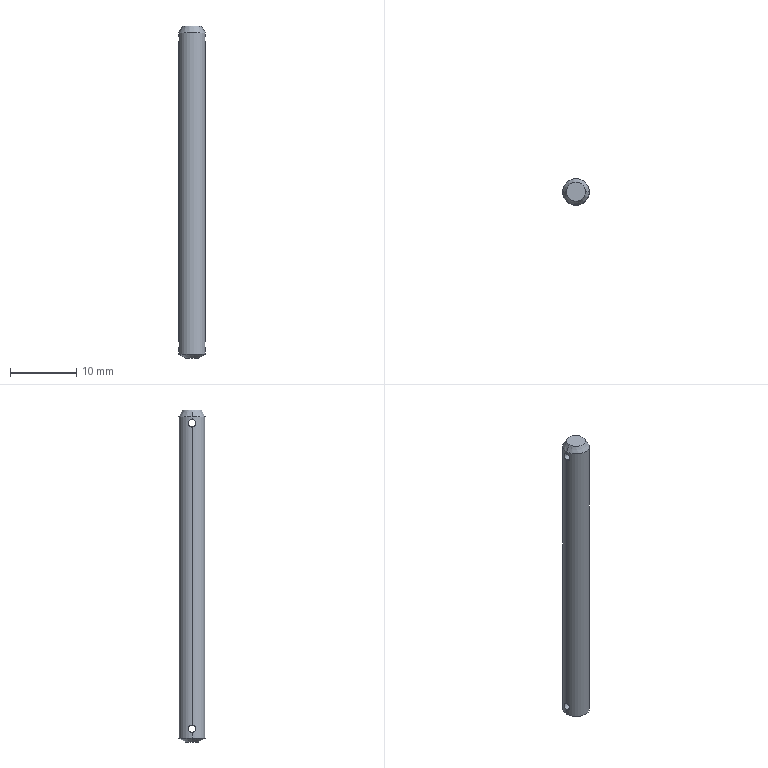Part | SolidWorks | features Chamfer 1, Cut 1, Extrusion 1 | 1 solid | 12 faces | box 4 x 4 x 50 mm | volume 613.938 mm3 | cylinder 6 | cone 4 | plane 2 | commonest cylinder face diameters 1.14 x4 4 x2
STEP:
#1=CARTESIAN_POINT('',(-2.,0.,-48.57));
#2=VERTEX_POINT('',#1);
#3=CARTESIAN_POINT('',(-2.,0.,-47.43));
#4=VERTEX_POINT('',#3);
#5=CARTESIAN_POINT('',(-2.,0.,-48.57));
#6=CARTESIAN_POINT('',(-2.,-0.1515,-48.57));
#7=CARTESIAN_POINT('',(-1.98,-0.2987,-48.508));
#8=CARTESIAN_POINT('',(-1.937,-0.5077,-48.298));
#9=CARTESIAN_POINT('',(-1.917,-0.5699,-48.15));
#10=CARTESIAN_POINT('',(-1.917,-0.5701,-47.851));
#11=CARTESIAN_POINT('',(-1.937,-0.5083,-47.702));
#12=CARTESIAN_POINT('',(-1.981,-0.2976,-47.492));
#13=CARTESIAN_POINT('',(-2.,-0.1493,-47.43));
#14=CARTESIAN_POINT('',(-2.,0.,-47.43));
#15=B_SPLINE_CURVE_WITH_KNOTS('',3,(#5,#6,#7,#8,#9,#10,#11,#12,#13,#14),.UNSPECIFIED.,.F.,.F.,(4,2,2,2,4),(0.,0.0004479,0.0008957,0.001344,0.001791),.UNSPECIFIED.);
#16=EDGE_CURVE('',#2,#4,#15,.T.);
#17=ORIENTED_EDGE('',*,*,#16,.T.);
#18=CARTESIAN_POINT('',(2.,0.,-47.43));
#19=VERTEX_POINT('',#18);
#20=CARTESIAN_POINT('',(-500.,0.,-47.43));
#21=DIRECTION('',(1.,0.,0.));
#22=VECTOR('',#21,1000.);
#23=LINE('',#20,#22);
#24=EDGE_CURVE('',#4,#19,#23,.T.);
#25=ORIENTED_EDGE('',*,*,#24,.T.);
#26=CARTESIAN_POINT('',(2.,0.,-48.57));
#27=VERTEX_POINT('',#26);
#28=CARTESIAN_POINT('',(2.,0.,-47.43));
#29=CARTESIAN_POINT('',(2.,-0.1493,-47.43));
#30=CARTESIAN_POINT('',(1.981,-0.2978,-47.492));
#31=CARTESIAN_POINT('',(1.937,-0.5081,-47.702));
#32=CARTESIAN_POINT('',(1.917,-0.57,-47.85));
#33=CARTESIAN_POINT('',(1.917,-0.57,-48.15));
#34=CARTESIAN_POINT('',(1.937,-0.5077,-48.298));
#35=CARTESIAN_POINT('',(1.98,-0.2988,-48.507));
#36=CARTESIAN_POINT('',(2.,-0.1515,-48.57));
#37=CARTESIAN_POINT('',(2.,0.,-48.57));
#38=B_SPLINE_CURVE_WITH_KNOTS('',3,(#28,#29,#30,#31,#32,#33,#34,#35,#36,#37),.UNSPECIFIED.,.F.,.F.,(4,2,2,2,4),(0.001791,0.002239,0.002687,0.003135,0.003582),.UNSPECIFIED.);
#39=EDGE_CURVE('',#19,#27,#38,.T.);
#40=ORIENTED_EDGE('',*,*,#39,.T.);
#41=CARTESIAN_POINT('',(-500.,0.,-48.57));
#42=DIRECTION('',(1.,0.,0.));
#43=VECTOR('',#42,1000.);
#44=LINE('',#41,#43);
#45=EDGE_CURVE('',#2,#27,#44,.T.);
#46=ORIENTED_EDGE('',*,*,#45,.F.);
#47=EDGE_LOOP('',(#17,#25,#40,#46));
#48=FACE_OUTER_BOUND('',#47,.T.);
#49=CARTESIAN_POINT('',(-500.,0.,-48.));
#50=DIRECTION('',(1.,0.,0.));
#51=DIRECTION('',(0.,0.,-1.));
#52=AXIS2_PLACEMENT_3D('',#49,#50,#51);
#53=CYLINDRICAL_SURFACE('',#52,0.57);
#54=ADVANCED_FACE('',(#48),#53,.F.);
#55=CARTESIAN_POINT('',(-2.,0.,-2.57));
#56=VERTEX_POINT('',#55);
#57=CARTESIAN_POINT('',(-2.,0.,-1.43));
#58=VERTEX_POINT('',#57);
#59=CARTESIAN_POINT('',(-2.,0.,-2.57));
#60=CARTESIAN_POINT('',(-2.,-0.1515,-2.57));
#61=CARTESIAN_POINT('',(-1.98,-0.2987,-2.508));
#62=CARTESIAN_POINT('',(-1.937,-0.5077,-2.298));
#63=CARTESIAN_POINT('',(-1.917,-0.5699,-2.15));
#64=CARTESIAN_POINT('',(-1.917,-0.5701,-1.851));
#65=CARTESIAN_POINT('',(-1.937,-0.5083,-1.702));
#66=CARTESIAN_POINT('',(-1.981,-0.2976,-1.492));
#67=CARTESIAN_POINT('',(-2.,-0.1493,-1.43));
#68=CARTESIAN_POINT('',(-2.,0.,-1.43));
#69=B_SPLINE_CURVE_WITH_KNOTS('',3,(#59,#60,#61,#62,#63,#64,#65,#66,#67,#68),.UNSPECIFIED.,.F.,.F.,(4,2,2,2,4),(0.,0.0004479,0.0008957,0.001344,0.001791),.UNSPECIFIED.);
#70=EDGE_CURVE('',#56,#58,#69,.T.);
#71=ORIENTED_EDGE('',*,*,#70,.T.);
#72=CARTESIAN_POINT('',(2.,0.,-1.43));
#73=VERTEX_POINT('',#72);
#74=CARTESIAN_POINT('',(-500.,0.,-1.43));
#75=DIRECTION('',(1.,0.,0.));
#76=VECTOR('',#75,1000.);
#77=LINE('',#74,#76);
#78=EDGE_CURVE('',#58,#73,#77,.T.);
#79=ORIENTED_EDGE('',*,*,#78,.T.);
#80=CARTESIAN_POINT('',(2.,0.,-2.57));
#81=VERTEX_POINT('',#80);
#82=CARTESIAN_POINT('',(2.,0.,-1.43));
#83=CARTESIAN_POINT('',(2.,-0.1493,-1.43));
#84=CARTESIAN_POINT('',(1.981,-0.2978,-1.492));
#85=CARTESIAN_POINT('',(1.937,-0.5081,-1.702));
#86=CARTESIAN_POINT('',(1.917,-0.57,-1.85));
#87=CARTESIAN_POINT('',(1.917,-0.57,-2.15));
#88=CARTESIAN_POINT('',(1.937,-0.5077,-2.298));
#89=CARTESIAN_POINT('',(1.98,-0.2988,-2.507));
#90=CARTESIAN_POINT('',(2.,-0.1515,-2.57));
#91=CARTESIAN_POINT('',(2.,0.,-2.57));
#92=B_SPLINE_CURVE_WITH_KNOTS('',3,(#82,#83,#84,#85,#86,#87,#88,#89,#90,#91),.UNSPECIFIED.,.F.,.F.,(4,2,2,2,4),(0.001791,0.002239,0.002687,0.003135,0.003582),.UNSPECIFIED.);
#93=EDGE_CURVE('',#73,#81,#92,.T.);
#94=ORIENTED_EDGE('',*,*,#93,.T.);
#95=CARTESIAN_POINT('',(-500.,0.,-2.57));
#96=DIRECTION('',(1.,0.,0.));
#97=VECTOR('',#96,1000.);
#98=LINE('',#95,#97);
#99=EDGE_CURVE('',#56,#81,#98,.T.);
#100=ORIENTED_EDGE('',*,*,#99,.F.);
#101=EDGE_LOOP('',(#71,#79,#94,#100));
#102=FACE_OUTER_BOUND('',#101,.T.);
#103=CARTESIAN_POINT('',(-500.,0.,-2.));
#104=DIRECTION('',(1.,0.,0.));
#105=DIRECTION('',(0.,0.,-1.));
#106=AXIS2_PLACEMENT_3D('',#103,#104,#105);
#107=CYLINDRICAL_SURFACE('',#106,0.57);
#108=ADVANCED_FACE('',(#102),#107,.F.);
#109=CARTESIAN_POINT('',(-1.,0.,-50.));
#110=VERTEX_POINT('',#109);
#111=CARTESIAN_POINT('',(1.,0.,-50.));
#112=VERTEX_POINT('',#111);
#113=CARTESIAN_POINT('',(0.,0.,-50.));
#114=DIRECTION('',(0.,0.,-1.));
#115=DIRECTION('',(1.,0.,0.));
#116=AXIS2_PLACEMENT_3D('',#113,#114,#115);
#117=CIRCLE('',#116,1.);
#118=EDGE_CURVE('',#110,#112,#117,.T.);
#119=ORIENTED_EDGE('',*,*,#118,.F.);
#120=CARTESIAN_POINT('',(-2.,0.,-49.423));
#121=VERTEX_POINT('',#120);
#122=CARTESIAN_POINT('',(-2.,0.,-49.423));
#123=DIRECTION('',(-0.866,0.,0.5));
#124=VECTOR('',#123,1000.);
#125=LINE('',#122,#124);
#126=EDGE_CURVE('',#110,#121,#125,.T.);
#127=ORIENTED_EDGE('',*,*,#126,.T.);
#128=CARTESIAN_POINT('',(2.,0.,-49.423));
#129=VERTEX_POINT('',#128);
#130=CARTESIAN_POINT('',(0.,0.,-49.423));
#131=DIRECTION('',(0.,0.,1.));
#132=DIRECTION('',(1.,0.,0.));
#133=AXIS2_PLACEMENT_3D('',#130,#131,#132);
#134=CIRCLE('',#133,2.);
#135=EDGE_CURVE('',#129,#121,#134,.T.);
#136=ORIENTED_EDGE('',*,*,#135,.F.);
#137=CARTESIAN_POINT('',(2.,0.,-49.423));
#138=DIRECTION('',(0.866,0.,0.5));
#139=VECTOR('',#138,1000.);
#140=LINE('',#137,#139);
#141=EDGE_CURVE('',#112,#129,#140,.T.);
#142=ORIENTED_EDGE('',*,*,#141,.F.);
#143=EDGE_LOOP('',(#119,#127,#136,#142));
#144=FACE_OUTER_BOUND('',#143,.T.);
#145=CARTESIAN_POINT('',(0.,0.,-49.423));
#146=DIRECTION('',(0.,0.,1.));
#147=DIRECTION('',(1.,0.,0.));
#148=AXIS2_PLACEMENT_3D('',#145,#146,#147);
#149=CONICAL_SURFACE('',#148,2.,1.047);
#150=ADVANCED_FACE('',(#144),#149,.T.);
#151=CARTESIAN_POINT('',(1.423,0.,0.));
#152=VERTEX_POINT('',#151);
#153=CARTESIAN_POINT('',(-1.423,0.,0.));
#154=VERTEX_POINT('',#153);
#155=CARTESIAN_POINT('',(0.,0.,0.));
#156=DIRECTION('',(0.,0.,1.));
#157=DIRECTION('',(1.,0.,0.));
#158=AXIS2_PLACEMENT_3D('',#155,#156,#157);
#159=CIRCLE('',#158,1.423);
#160=EDGE_CURVE('',#152,#154,#159,.T.);
#161=ORIENTED_EDGE('',*,*,#160,.F.);
#162=CARTESIAN_POINT('',(2.,0.,-1.));
#163=VERTEX_POINT('',#162);
#164=CARTESIAN_POINT('',(1.423,0.,0.));
#165=DIRECTION('',(0.5,0.,-0.866));
#166=VECTOR('',#165,1000.);
#167=LINE('',#164,#166);
#168=EDGE_CURVE('',#152,#163,#167,.T.);
#169=ORIENTED_EDGE('',*,*,#168,.T.);
#170=CARTESIAN_POINT('',(-2.,0.,-1.));
#171=VERTEX_POINT('',#170);
#172=CARTESIAN_POINT('',(0.,0.,-1.));
#173=DIRECTION('',(0.,0.,-1.));
#174=DIRECTION('',(1.,0.,0.));
#175=AXIS2_PLACEMENT_3D('',#172,#173,#174);
#176=CIRCLE('',#175,2.);
#177=EDGE_CURVE('',#171,#163,#176,.T.);
#178=ORIENTED_EDGE('',*,*,#177,.F.);
#179=CARTESIAN_POINT('',(-1.423,0.,0.));
#180=DIRECTION('',(-0.5,0.,-0.866));
#181=VECTOR('',#180,1000.);
#182=LINE('',#179,#181);
#183=EDGE_CURVE('',#154,#171,#182,.T.);
#184=ORIENTED_EDGE('',*,*,#183,.F.);
#185=EDGE_LOOP('',(#161,#169,#178,#184));
#186=FACE_OUTER_BOUND('',#185,.T.);
#187=CARTESIAN_POINT('',(0.,0.,0.));
#188=DIRECTION('',(0.,0.,-1.));
#189=DIRECTION('',(-1.,0.,0.));
#190=AXIS2_PLACEMENT_3D('',#187,#188,#189);
#191=CONICAL_SURFACE('',#190,1.423,0.5236);
#192=ADVANCED_FACE('',(#186),#191,.T.);
#193=ORIENTED_EDGE('',*,*,#135,.T.);
#194=CARTESIAN_POINT('',(-2.,0.,-50.));
#195=DIRECTION('',(0.,0.,1.));
#196=VECTOR('',#195,1000.);
#197=LINE('',#194,#196);
#198=EDGE_CURVE('',#121,#2,#197,.T.);
#199=ORIENTED_EDGE('',*,*,#198,.T.);
#200=CARTESIAN_POINT('',(-2.,0.,-47.43));
#201=CARTESIAN_POINT('',(-2.,0.1493,-47.43));
#202=CARTESIAN_POINT('',(-1.981,0.2978,-47.492));
#203=CARTESIAN_POINT('',(-1.937,0.5081,-47.702));
#204=CARTESIAN_POINT('',(-1.917,0.57,-47.85));
#205=CARTESIAN_POINT('',(-1.917,0.57,-48.15));
#206=CARTESIAN_POINT('',(-1.937,0.5077,-48.298));
#207=CARTESIAN_POINT('',(-1.98,0.2988,-48.507));
#208=CARTESIAN_POINT('',(-2.,0.1515,-48.57));
#209=CARTESIAN_POINT('',(-2.,0.,-48.57));
#210=B_SPLINE_CURVE_WITH_KNOTS('',3,(#200,#201,#202,#203,#204,#205,#206,#207,#208,#209),.UNSPECIFIED.,.F.,.F.,(4,2,2,2,4),(0.001791,0.002239,0.002687,0.003135,0.003582),.UNSPECIFIED.);
#211=EDGE_CURVE('',#4,#2,#210,.T.);
#212=ORIENTED_EDGE('',*,*,#211,.F.);
#213=CARTESIAN_POINT('',(-2.,0.,-50.));
#214=DIRECTION('',(0.,0.,1.));
#215=VECTOR('',#214,1000.);
#216=LINE('',#213,#215);
#217=EDGE_CURVE('',#4,#56,#216,.T.);
#218=ORIENTED_EDGE('',*,*,#217,.T.);
#219=CARTESIAN_POINT('',(-2.,0.,-1.43));
#220=CARTESIAN_POINT('',(-2.,0.1493,-1.43));
#221=CARTESIAN_POINT('',(-1.981,0.2978,-1.492));
#222=CARTESIAN_POINT('',(-1.937,0.5081,-1.702));
#223=CARTESIAN_POINT('',(-1.917,0.57,-1.85));
#224=CARTESIAN_POINT('',(-1.917,0.57,-2.15));
#225=CARTESIAN_POINT('',(-1.937,0.5077,-2.298));
#226=CARTESIAN_POINT('',(-1.98,0.2988,-2.507));
#227=CARTESIAN_POINT('',(-2.,0.1515,-2.57));
#228=CARTESIAN_POINT('',(-2.,0.,-2.57));
#229=B_SPLINE_CURVE_WITH_KNOTS('',3,(#219,#220,#221,#222,#223,#224,#225,#226,#227,#228),.UNSPECIFIED.,.F.,.F.,(4,2,2,2,4),(0.001791,0.002239,0.002687,0.003135,0.003582),.UNSPECIFIED.);
#230=EDGE_CURVE('',#58,#56,#229,.T.);
#231=ORIENTED_EDGE('',*,*,#230,.F.);
#232=CARTESIAN_POINT('',(-2.,0.,-50.));
#233=DIRECTION('',(0.,0.,1.));
#234=VECTOR('',#233,1000.);
#235=LINE('',#232,#234);
#236=EDGE_CURVE('',#58,#171,#235,.T.);
#237=ORIENTED_EDGE('',*,*,#236,.T.);
#238=ORIENTED_EDGE('',*,*,#177,.T.);
#239=CARTESIAN_POINT('',(2.,0.,-50.));
#240=DIRECTION('',(0.,0.,1.));
#241=VECTOR('',#240,1000.);
#242=LINE('',#239,#241);
#243=EDGE_CURVE('',#73,#163,#242,.T.);
#244=ORIENTED_EDGE('',*,*,#243,.F.);
#245=CARTESIAN_POINT('',(2.,0.,-2.57));
#246=CARTESIAN_POINT('',(2.,0.1515,-2.57));
#247=CARTESIAN_POINT('',(1.98,0.2987,-2.508));
#248=CARTESIAN_POINT('',(1.937,0.5077,-2.298));
#249=CARTESIAN_POINT('',(1.917,0.5699,-2.15));
#250=CARTESIAN_POINT('',(1.917,0.5701,-1.851));
#251=CARTESIAN_POINT('',(1.937,0.5083,-1.702));
#252=CARTESIAN_POINT('',(1.981,0.2976,-1.492));
#253=CARTESIAN_POINT('',(2.,0.1493,-1.43));
#254=CARTESIAN_POINT('',(2.,0.,-1.43));
#255=B_SPLINE_CURVE_WITH_KNOTS('',3,(#245,#246,#247,#248,#249,#250,#251,#252,#253,#254),.UNSPECIFIED.,.F.,.F.,(4,2,2,2,4),(0.,0.0004479,0.0008957,0.001344,0.001791),.UNSPECIFIED.);
#256=EDGE_CURVE('',#81,#73,#255,.T.);
#257=ORIENTED_EDGE('',*,*,#256,.F.);
#258=CARTESIAN_POINT('',(2.,0.,-50.));
#259=DIRECTION('',(0.,0.,1.));
#260=VECTOR('',#259,1000.);
#261=LINE('',#258,#260);
#262=EDGE_CURVE('',#19,#81,#261,.T.);
#263=ORIENTED_EDGE('',*,*,#262,.F.);
#264=CARTESIAN_POINT('',(2.,0.,-48.57));
#265=CARTESIAN_POINT('',(2.,0.1515,-48.57));
#266=CARTESIAN_POINT('',(1.98,0.2987,-48.508));
#267=CARTESIAN_POINT('',(1.937,0.5077,-48.298));
#268=CARTESIAN_POINT('',(1.917,0.5699,-48.15));
#269=CARTESIAN_POINT('',(1.917,0.5701,-47.851));
#270=CARTESIAN_POINT('',(1.937,0.5083,-47.702));
#271=CARTESIAN_POINT('',(1.981,0.2976,-47.492));
#272=CARTESIAN_POINT('',(2.,0.1493,-47.43));
#273=CARTESIAN_POINT('',(2.,0.,-47.43));
#274=B_SPLINE_CURVE_WITH_KNOTS('',3,(#264,#265,#266,#267,#268,#269,#270,#271,#272,#273),.UNSPECIFIED.,.F.,.F.,(4,2,2,2,4),(0.,0.0004479,0.0008957,0.001344,0.001791),.UNSPECIFIED.);
#275=EDGE_CURVE('',#27,#19,#274,.T.);
#276=ORIENTED_EDGE('',*,*,#275,.F.);
#277=CARTESIAN_POINT('',(2.,0.,-50.));
#278=DIRECTION('',(0.,0.,1.));
#279=VECTOR('',#278,1000.);
#280=LINE('',#277,#279);
#281=EDGE_CURVE('',#129,#27,#280,.T.);
#282=ORIENTED_EDGE('',*,*,#281,.F.);
#283=EDGE_LOOP('',(#193,#199,#212,#218,#231,#237,#238,#244,#257,#263,#276,#282));
#284=FACE_OUTER_BOUND('',#283,.T.);
#285=CARTESIAN_POINT('',(0.,0.,-50.));
#286=DIRECTION('',(0.,0.,1.));
#287=DIRECTION('',(1.,0.,0.));
#288=AXIS2_PLACEMENT_3D('',#285,#286,#287);
#289=CYLINDRICAL_SURFACE('',#288,2.);
#290=ADVANCED_FACE('',(#284),#289,.T.);
#291=ORIENTED_EDGE('',*,*,#198,.F.);
#292=CARTESIAN_POINT('',(0.,0.,-49.423));
#293=DIRECTION('',(0.,0.,1.));
#294=DIRECTION('',(1.,0.,0.));
#295=AXIS2_PLACEMENT_3D('',#292,#293,#294);
#296=CIRCLE('',#295,2.);
#297=EDGE_CURVE('',#121,#129,#296,.T.);
#298=ORIENTED_EDGE('',*,*,#297,.T.);
#299=ORIENTED_EDGE('',*,*,#281,.T.);
#300=ORIENTED_EDGE('',*,*,#39,.F.);
#301=ORIENTED_EDGE('',*,*,#262,.T.);
#302=ORIENTED_EDGE('',*,*,#93,.F.);
#303=ORIENTED_EDGE('',*,*,#243,.T.);
#304=CARTESIAN_POINT('',(0.,0.,-1.));
#305=DIRECTION('',(0.,0.,-1.));
#306=DIRECTION('',(1.,0.,0.));
#307=AXIS2_PLACEMENT_3D('',#304,#305,#306);
#308=CIRCLE('',#307,2.);
#309=EDGE_CURVE('',#163,#171,#308,.T.);
#310=ORIENTED_EDGE('',*,*,#309,.T.);
#311=ORIENTED_EDGE('',*,*,#236,.F.);
#312=ORIENTED_EDGE('',*,*,#70,.F.);
#313=ORIENTED_EDGE('',*,*,#217,.F.);
#314=ORIENTED_EDGE('',*,*,#16,.F.);
#315=EDGE_LOOP('',(#291,#298,#299,#300,#301,#302,#303,#310,#311,#312,#313,#314));
#316=FACE_OUTER_BOUND('',#315,.T.);
#317=CARTESIAN_POINT('',(0.,0.,-50.));
#318=DIRECTION('',(0.,0.,1.));
#319=DIRECTION('',(1.,0.,0.));
#320=AXIS2_PLACEMENT_3D('',#317,#318,#319);
#321=CYLINDRICAL_SURFACE('',#320,2.);
#322=ADVANCED_FACE('',(#316),#321,.T.);
#323=CARTESIAN_POINT('',(0.,0.,-50.));
#324=DIRECTION('',(0.,0.,-1.));
#325=DIRECTION('',(1.,0.,0.));
#326=AXIS2_PLACEMENT_3D('',#323,#324,#325);
#327=CIRCLE('',#326,1.);
#328=EDGE_CURVE('',#112,#110,#327,.T.);
#329=ORIENTED_EDGE('',*,*,#328,.T.);
#330=ORIENTED_EDGE('',*,*,#118,.T.);
#331=EDGE_LOOP('',(#329,#330));
#332=FACE_OUTER_BOUND('',#331,.T.);
#333=CARTESIAN_POINT('',(0.,0.,-50.));
#334=DIRECTION('',(0.,0.,1.));
#335=DIRECTION('',(1.,0.,0.));
#336=AXIS2_PLACEMENT_3D('',#333,#334,#335);
#337=PLANE('',#336);
#338=ADVANCED_FACE('',(#332),#337,.F.);
#339=CARTESIAN_POINT('',(0.,0.,0.));
#340=DIRECTION('',(0.,0.,1.));
#341=DIRECTION('',(1.,0.,0.));
#342=AXIS2_PLACEMENT_3D('',#339,#340,#341);
#343=CIRCLE('',#342,1.423);
#344=EDGE_CURVE('',#154,#152,#343,.T.);
#345=ORIENTED_EDGE('',*,*,#344,.T.);
#346=ORIENTED_EDGE('',*,*,#160,.T.);
#347=EDGE_LOOP('',(#345,#346));
#348=FACE_OUTER_BOUND('',#347,.T.);
#349=CARTESIAN_POINT('',(0.,0.,0.));
#350=DIRECTION('',(0.,0.,1.));
#351=DIRECTION('',(1.,0.,0.));
#352=AXIS2_PLACEMENT_3D('',#349,#350,#351);
#353=PLANE('',#352);
#354=ADVANCED_FACE('',(#348),#353,.T.);
#355=ORIENTED_EDGE('',*,*,#168,.F.);
#356=ORIENTED_EDGE('',*,*,#344,.F.);
#357=ORIENTED_EDGE('',*,*,#183,.T.);
#358=ORIENTED_EDGE('',*,*,#309,.F.);
#359=EDGE_LOOP('',(#355,#356,#357,#358));
#360=FACE_OUTER_BOUND('',#359,.T.);
#361=CARTESIAN_POINT('',(0.,0.,0.));
#362=DIRECTION('',(0.,0.,-1.));
#363=DIRECTION('',(-1.,0.,0.));
#364=AXIS2_PLACEMENT_3D('',#361,#362,#363);
#365=CONICAL_SURFACE('',#364,1.423,0.5236);
#366=ADVANCED_FACE('',(#360),#365,.T.);
#367=ORIENTED_EDGE('',*,*,#126,.F.);
#368=ORIENTED_EDGE('',*,*,#328,.F.);
#369=ORIENTED_EDGE('',*,*,#141,.T.);
#370=ORIENTED_EDGE('',*,*,#297,.F.);
#371=EDGE_LOOP('',(#367,#368,#369,#370));
#372=FACE_OUTER_BOUND('',#371,.T.);
#373=CARTESIAN_POINT('',(0.,0.,-49.423));
#374=DIRECTION('',(0.,0.,1.));
#375=DIRECTION('',(1.,0.,0.));
#376=AXIS2_PLACEMENT_3D('',#373,#374,#375);
#377=CONICAL_SURFACE('',#376,2.,1.047);
#378=ADVANCED_FACE('',(#372),#377,.T.);
#379=ORIENTED_EDGE('',*,*,#78,.F.);
#380=ORIENTED_EDGE('',*,*,#230,.T.);
#381=ORIENTED_EDGE('',*,*,#99,.T.);
#382=ORIENTED_EDGE('',*,*,#256,.T.);
#383=EDGE_LOOP('',(#379,#380,#381,#382));
#384=FACE_OUTER_BOUND('',#383,.T.);
#385=CARTESIAN_POINT('',(-500.,0.,-2.));
#386=DIRECTION('',(1.,0.,0.));
#387=DIRECTION('',(0.,0.,-1.));
#388=AXIS2_PLACEMENT_3D('',#385,#386,#387);
#389=CYLINDRICAL_SURFACE('',#388,0.57);
#390=ADVANCED_FACE('',(#384),#389,.F.);
#391=ORIENTED_EDGE('',*,*,#24,.F.);
#392=ORIENTED_EDGE('',*,*,#211,.T.);
#393=ORIENTED_EDGE('',*,*,#45,.T.);
#394=ORIENTED_EDGE('',*,*,#275,.T.);
#395=EDGE_LOOP('',(#391,#392,#393,#394));
#396=FACE_OUTER_BOUND('',#395,.T.);
#397=CARTESIAN_POINT('',(-500.,0.,-48.));
#398=DIRECTION('',(1.,0.,0.));
#399=DIRECTION('',(0.,0.,-1.));
#400=AXIS2_PLACEMENT_3D('',#397,#398,#399);
#401=CYLINDRICAL_SURFACE('',#400,0.57);
#402=ADVANCED_FACE('',(#396),#401,.F.);
#403=CLOSED_SHELL('',(#54,#108,#150,#192,#290,#322,#338,#354,#366,#378,#390,#402));
#404=MANIFOLD_SOLID_BREP('',#403);
#405=CARTESIAN_POINT('',(0.,0.,0.));
#406=DIRECTION('',(0.,0.,1.));
#407=DIRECTION('',(1.,0.,0.));
#408=AXIS2_PLACEMENT_3D('',#405,#406,#407);
#409=(LENGTH_UNIT()NAMED_UNIT(*)SI_UNIT(.MILLI.,.METRE.));
#410=UNCERTAINTY_MEASURE_WITH_UNIT(LENGTH_MEASURE(0.00001),#409,'','');
#411=(NAMED_UNIT(*)PLANE_ANGLE_UNIT()SI_UNIT($,.RADIAN.));
#412=(NAMED_UNIT(*)SI_UNIT($,.STERADIAN.)SOLID_ANGLE_UNIT());
#413=(GEOMETRIC_REPRESENTATION_CONTEXT(3)GLOBAL_UNCERTAINTY_ASSIGNED_CONTEXT((#410))GLOBAL_UNIT_ASSIGNED_CONTEXT((#409,#411,#412))REPRESENTATION_CONTEXT('',''));
#414=ADVANCED_BREP_SHAPE_REPRESENTATION('',(#404,#408),#413);